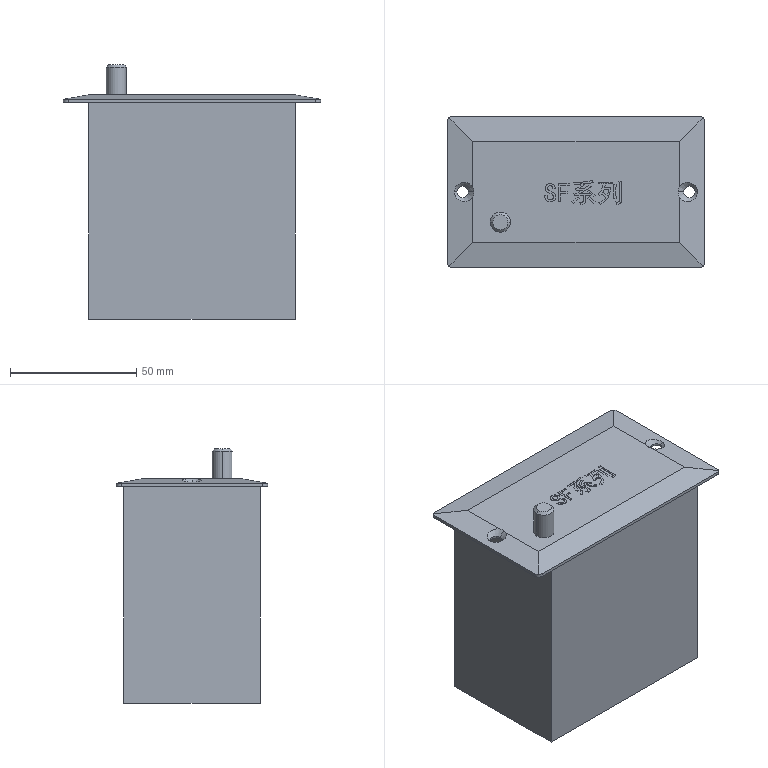Part | STEP file | QA-SF系列调整器-1 | 1 solid | 141 faces | box 102 x 60 x 101 mm | volume 397007 mm3 | spline 69 | plane 56 | cylinder 10 | cone 6 | commonest cylinder face diameters 4 x4 4.5 x4 8 x2